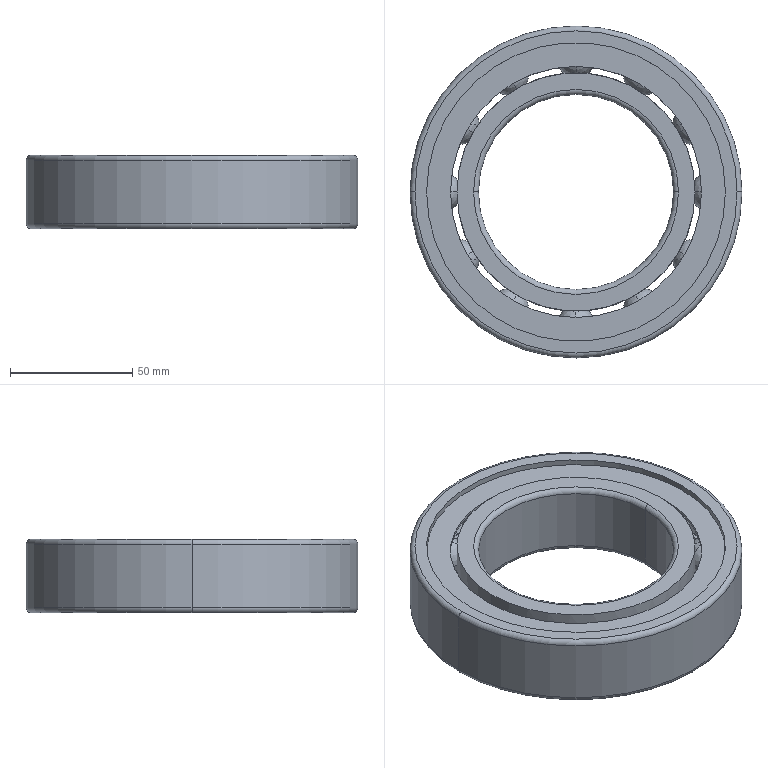Part | SolidWorks | features BaseBody 1 | 1 solid | 296 faces | box 136 x 136 x 30 mm | volume 182204 mm3 | sphere 196 | torus 44 | plane 32 | cylinder 24 | commonest cylinder face diameters 122.4 x8 97.6 x4 102.88 x4 80 x2 108.69 x2 111.31 x2